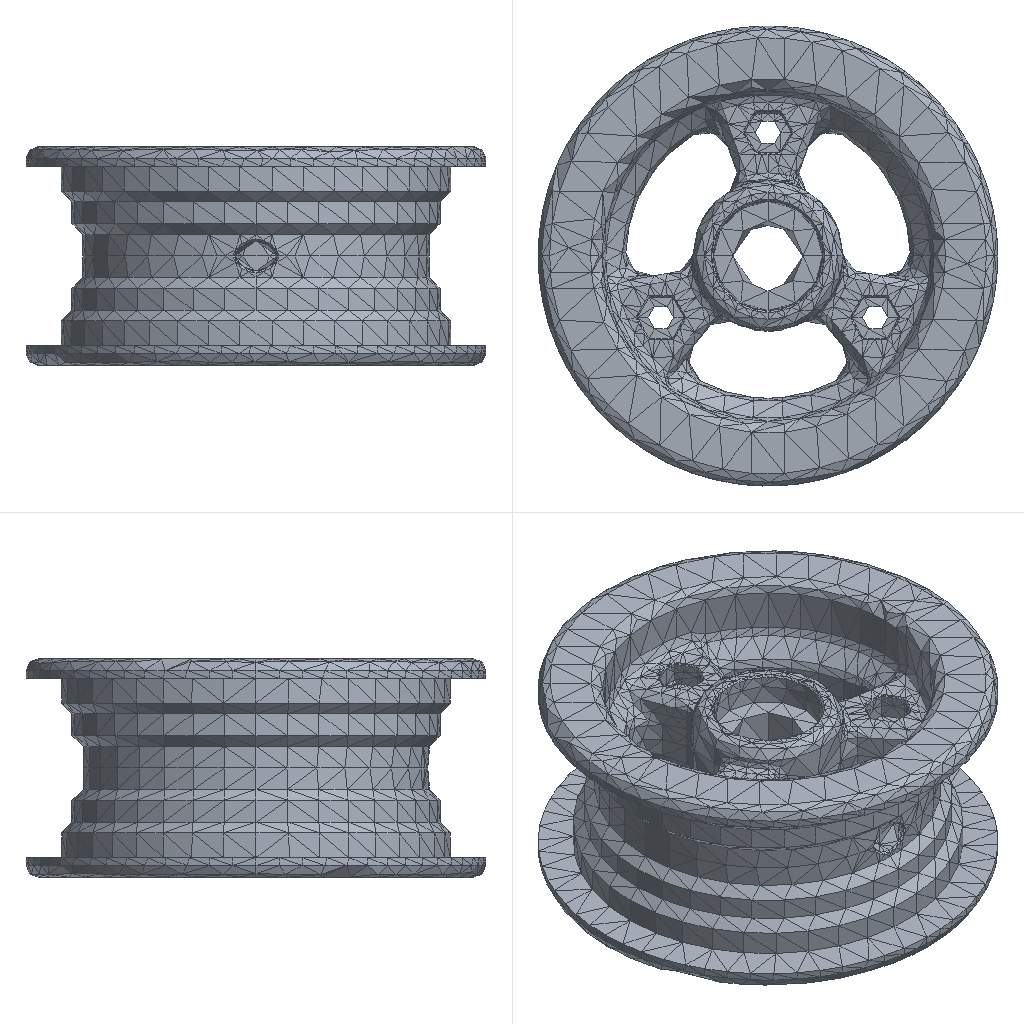Simulation study | ansys workbench
Ansys APDL input file, long lists of numbers shortened:
/batch
/config,noeldb,1     ! force off writing results to database
*get,_wallstrt,active,,time,wall
! ANSYS input file written by Workbench version 2022 R1
! File used for geometry attach:
/title,wbnew--____ (G5)
! ****** Begin Custom Load Command Snippet ******
/COM, ACT Extensions:
/COM,     LSDYNA, 2021.1
/COM,
! ****** End   Custom Load Command Snippet ******
*DIM,_wb_ProjectScratch_dir,string,248
_wb_ProjectScratch_dir(1) = ''
*DIM,_wb_SolverFiles_dir,string,248
_wb_SolverFiles_dir(1) = ''
*DIM,_wb_userfiles_dir,string,248
_wb_userfiles_dir(1) = ''
/com,--- Data in consistent NMM units. See Solving Units in the help system for more information.
/units,MPA
/nopr
/wb,file,start              !  signify a WB generated input file
/prep7
! Turn off shape checking because checks already performed inside WB mesher.
! See help system for more information.
SHPP,OFF,,NOWARN
/nolist
etcon,set             ! allow ANSYS to choose best KEYOP's for 180x elements, resets any applicable keyopt to MAPDL defaults
/com,*********** Nodes for the whole assembly ***********
nblock,3,,26501
(1i9,3e20.9e3)
        1    -4.560694183E+01    -3.299351067E+01     2.580641396E+01
! (24091 more lines like these left out)
-1
/com,*********** Nodes for all Remote Points ***********
nblock,3
(1i9,3e20.9e3)
    24093    -5.164900630E+01     1.110982665E+01     2.580641396E+01
-1
/wb,elem,start            !  set before creation of elements
/com,*********** Elements for Body 1 "Wheel Hub|NONE" ***********
et,1,187
eblock,19,solid,,6435
(19i9)
        1        1        1        1        0        0        0        0       10        0        1     1626     1629     1961     1928    11164    11185    11170    11169
! (12869 more lines like these left out)
-1
/com,*********** Elements for Body 2 "Wheel Hub|NONE[2]" ***********
et,2,187
eblock,19,solid,,6435
(19i9)
        2        2        2        2        0        0        0        0       10        0     6436    13672    13675    14007    13974    23210    23231    23216    23215
! (12869 more lines like these left out)
-1
/wb,elem,end               !  done creating elements
/com,*********** Send User Defined Coordinate System(s) ***********
csys,0
toffst,273.15,  ! Temperature offset from absolute zero
/com,*********** Set Reference Temperature ***********
tref,22.
/wb,mat,start              !  starting to send materials
/com,*********** Send Materials ***********
Temperature = 'TEMP' ! Temperature
MP,DENS,1,7.85e-09,	! tonne mm^-3
MP,ALPX,1,1.2e-05,	! C^-1
MP,C,1,434000000,	! mm^2 s^-2 C^-1
MP,KXX,1,60.5,	! tonne mm s^-3 C^-1
MP,RSVX,1,0.00017,	! ohm mm
MP,EX,1,200000,	! tonne s^-2 mm^-1
MP,NUXY,1,0.3,
MP,MURX,1,10000,
Temperature = 'TEMP' ! Temperature
MP,DENS,2,7.85e-09,	! tonne mm^-3
MP,ALPX,2,1.2e-05,	! C^-1
MP,C,2,434000000,	! mm^2 s^-2 C^-1
MP,KXX,2,60.5,	! tonne mm s^-3 C^-1
MP,RSVX,2,0.00017,	! ohm mm
MP,EX,2,200000,	! tonne s^-2 mm^-1
MP,NUXY,2,0.3,
MP,MURX,2,10000,
/wb,mat,end                !  done sending materials
!************************* Model Summary ********************
!Wheel Hub|NONE,	6061,	matid,	1
!Wheel Hub|NONE[2],	6061,	matid,	2
!************************* End Model Summary ********************
! get the diagonal of the bounding box. Needed later for other things
*get,_xmin,node,,mnloc,x
*get,_ymin,node,,mnloc,y
*get,_zmin,node,,mnloc,z
*get,_xmax,node,,mxloc,x
*get,_ymax,node,,mxloc,y
*get,_zmax,node,,mxloc,z
_ASMDIAG=(_xmax-_xmin)*(_xmax-_xmin)+(_ymax-_ymin)*(_ymax-_ymin)+(_zmax-_zmin)*(_zmax-_zmin)
_ASMDIAG=SQRT(_ASMDIAG)
/wb,contact,start          !  starting to send contact
/com,*********** Create Contact "接触区域" ***********
/com,            Real Constant Set For Above Contact Is 4 & 3
*set,tid,4
*set,cid,3
r,tid
r,cid
et,tid,170
et,cid,174
eblock,10,,,300
(15i9)
    19468        4        4        4        0       39       44       45       45     2204     2244       45     2205
! (299 more lines like these left out)
-1
eblock,10,,,300
(15i9)
    19768        3        3        3        0       39       44       45       45     2204     2244       45     2205
! (299 more lines like these left out)
-1
eblock,10,,,300
(15i9)
    20068        3        4        3        0    12105    13001    13171    13171    14383    20564    13171    14384
! (299 more lines like these left out)
-1
eblock,10,,,300
(15i9)
    20368        4        3        4        0    12105    13001    13171    13171    14383    20564    13171    14384
! (299 more lines like these left out)
-1
keyo,cid,8,2               ! auto create asymmetric contact (from Program Controlled setting)
keyo,cid,10,0              ! adjust contact stiffness each NR iteration (from Program Controlled setting)
keyo,cid,12,5              ! bonded always
keyo,cid,18,1              ! small sliding turned on by application
keyo,cid,2,0               ! augmented Lagrange (from Program Controlled setting)
keyo,cid,4,0               ! on Gauss point (from Program Controlled setting)
keyo,cid,9,1               ! ignore initial gaps/penetration
keyo,cid,7,0               ! No Prediction
rmod,tid,3,10.      ! FKN
rmod,tid,5,0.       ! ICONT
rmod,tid,6,0.       ! PINB
rmod,tid,10,0.      ! CNOF
rmod,tid,12,0.      ! FKT
rmod,tid,36,29      ! WB DSID
rmod,cid,3,10.      ! FKN
rmod,cid,5,0.       ! ICONT
rmod,cid,6,0.       ! PINB
rmod,cid,10,0.      ! CNOF
rmod,cid,12,0.      ! FKT
rmod,cid,36,29      ! WB DSID
nsel,all
esel,all
/wb,contact,end            !  done creating contacts
/golist
/wb,load,start             !  starting to send loads
/com,*********** Fixed Supports ***********
CMBLOCK,_FIXEDSU,NODE,      128
(8i10)
       823       824       825       826       827       828       829       830
! (15 more lines like these left out)
cmsel,s,_FIXEDSU
d,all,all
nsel,all
/com,*********** Create Remote Point "内部远程点" ***********
! -------- Remote Point Used by "力矩" --------
*set,tid,6
*set,cid,5
et,cid,174
et,tid,170
keyo,tid,2,1               ! Don't fix the pilot node
keyo,tid,4,111111
keyo,cid,12,5              ! Bonded Contact
keyo,cid,4,1               ! Deformable RBE3 style load
keyo,cid,2,2               ! MPC style contact
eblock,10,,,202
(15i9)
    20668        5        5        5        0      225      510      578      578     3496     5665      578     3497
! (201 more lines like these left out)
-1
*set,_npilot,24093
_npilot40=_npilot
type,tid
mat ,cid
real,cid
tshape,pilo
en,20870,_npilot
tshape
/com,*********** Construct Moment Using Remote Attachment ***********
/gst,on,on
fini
*get,_numnode,node,0,count
*get,_numelem,elem,0,count
*get, _MAXELEMNUM, elem, 0, NUM, MAX
*get, _MAXNODENUM, node, 0, NUM, MAX
*get, _MAXELEMTYPE, etyp, 0, NUM, MAX
*get, _MAXREALCONST, real, 0, NUM, MAX
/go
/wb,load,end               !  done creating loads
/com,--- Number of total nodes = %_numnode%
/com,--- Number of contact elements = 1402
/com,--- Number of spring elements = 0
/com,--- Number of bearing elements = 0
/com,--- Number of solid elements = 12870
/com,--- Number of condensed parts = 0
/com,--- Number of total elements = %_numelem%
*get,_wallbsol,active,,time,wall
/com,****************************************************************************
/com,*************************    SOLUTION       ********************************
/com,****************************************************************************
/solu
antype,0                   ! static analysis
_thickRatio=  1     ! Ratio of thick parts in the model
eqsl,pcg,1e-8,,,,,,1
cntr,print,1               ! print out contact info and also make no initial contact an error
dmpoption,emat,no             ! Don't combine emat file for DANSYS
dmpoption,esav,no             ! Don't combine esav file for DANSYS
nldiag,cont,iter           ! print out contact info each equilibrium iteration
rescontrol,,none                 ! Do not keep any restart files
/com,****************************************************
/com,******************* SOLVE FOR LS 1 OF 1 ****************
nsel,s,node,,24093
f,all,mx,0.
f,all,my,0.
f,all,mz,50000.
nsel,all
/nopr
/gopr
nsub,1,1,1
time,1.
outres,erase
outres,all,none
outres,nsol,all,
outres,rsol,all
outres,eangl,all
outres,etmp,all
outres,veng,all
outres,strs,all,
outres,epel,all,
outres,eppl,all,
outres,cont,all,
! *********** WB SOLVE COMMAND ***********
! check interactive state
*get,ANSINTER_,active,,int
*if,ANSINTER_,ne,0,then
/eof
*endif
solve
/com *************** Write FE CONNECTORS *********
CEWRITE,file,ce,,INTE
/com,****************************************************
/com,*************** FINISHED SOLVE FOR LS 1 *************
*get,_wallasol,active,,time,wall
/nopr
*get,_numnode,node,0,count
*get,_numelem,elem,0,count
*get, _MAXELEMNUM, elem, 0, NUM, MAX
*get, _MAXNODENUM, node, 0, NUM, MAX,,,INTERNAL
*get, _MAXELEMTYPE, etyp, 0, NUM, MAX
*get, _MAXREALCONST, real, 0, NUM, MAX
/gopr
*get,_PCGITER,active,,solu,cgiter
/post1
xmlo,ENCODING,ISO-8859-1
xmlo,parm
/xml,parm,xml
fini
/gopr
*get,_walldone,active,,time,wall
_preptime=(_wallbsol-_wallstrt)*3600
_solvtime=(_wallasol-_wallbsol)*3600
_posttime=(_walldone-_wallasol)*3600
_totaltim=(_walldone-_wallstrt)*3600
*get,_dlbratio,active,0,solu,dlbr
*get,_combtime,active,0,solu,comb
*get,_ssmode,active,0,solu,ssmm
*get,_ndofs,active,0,solu,ndof
*get,_sol_end_time,active,0,set,time
*if,_sol_end_time,eq,1.,then
/fclean				!clean distributed files
*endif
/com,--- Total number of nodes = %_numnode%
/com,--- Total number of elements = %_numelem%
/com,--- Element load balance ratio = %_dlbratio%
/com,--- Time to combine distributed files = %_combtime%
/com,--- Sparse memory mode = %_ssmode%
/com,--- Number of DOF = %_ndofs%
/wb,file,end               ! done with WB generated input